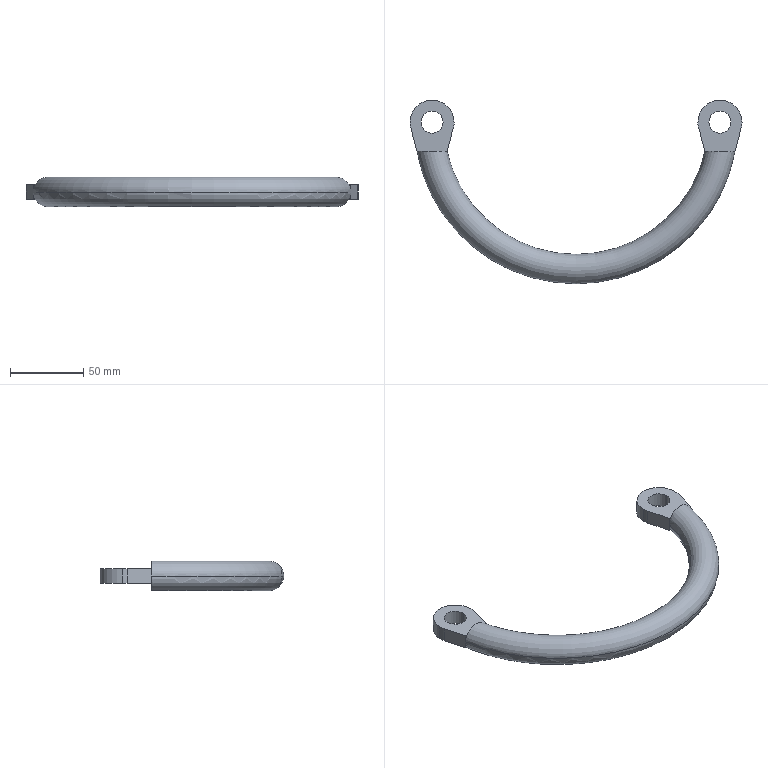Part | SolidWorks | features ICE 2, MirrorPattern 1, Sweep 1 | 1 solid | 36 faces | box 225.916 x 125 x 20 mm | volume 44773 mm3 | plane 22 | cylinder 10 | torus 4 | commonest cylinder face diameters 30 x6 15 x4